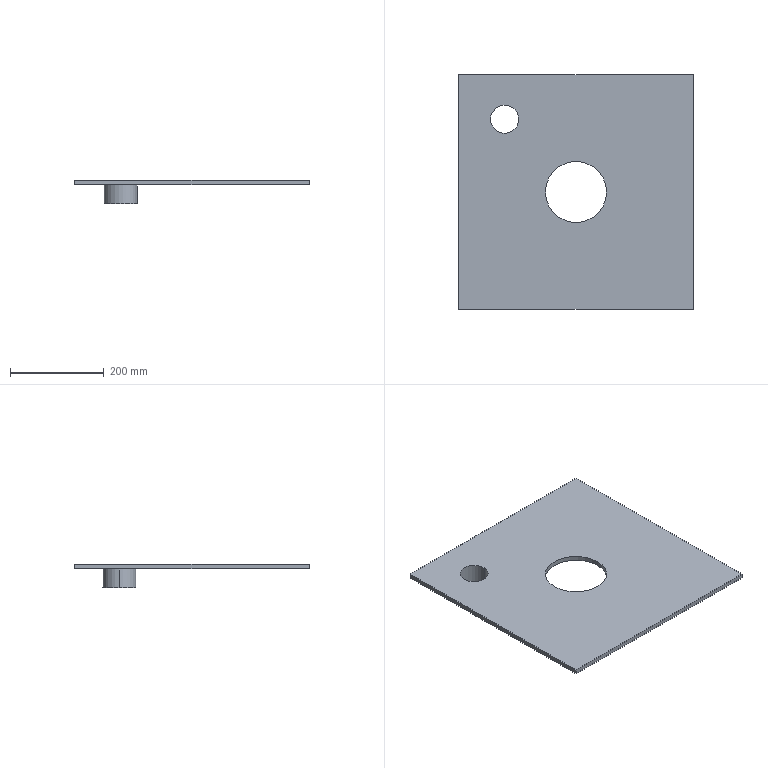Part | SolidWorks | features Extrusion 1, ICE 1 | 1 solid | 13 faces | box 500 x 500 x 50 mm | volume 2380238 mm3 | plane 7 | cylinder 6 | commonest cylinder face diameters 59.914 x2 70 x2 130 x2
STEP:
#1=CARTESIAN_POINT('',(67.956,404.852,-40.));
#2=VERTEX_POINT('',#1);
#3=CARTESIAN_POINT('',(127.871,404.852,-40.));
#4=VERTEX_POINT('',#3);
#5=CARTESIAN_POINT('',(97.914,404.852,-40.));
#6=DIRECTION('',(0.,0.,1.));
#7=DIRECTION('',(1.,0.,0.));
#8=AXIS2_PLACEMENT_3D('',#5,#6,#7);
#9=CIRCLE('',#8,29.957);
#10=EDGE_CURVE('',#2,#4,#9,.T.);
#11=ORIENTED_EDGE('',*,*,#10,.F.);
#12=CARTESIAN_POINT('',(67.956,404.852,10.));
#13=VERTEX_POINT('',#12);
#14=CARTESIAN_POINT('',(67.956,404.852,-40.));
#15=DIRECTION('',(0.,0.,1.));
#16=VECTOR('',#15,1000.);
#17=LINE('',#14,#16);
#18=EDGE_CURVE('',#2,#13,#17,.T.);
#19=ORIENTED_EDGE('',*,*,#18,.T.);
#20=CARTESIAN_POINT('',(127.871,404.852,10.));
#21=VERTEX_POINT('',#20);
#22=CARTESIAN_POINT('',(97.914,404.852,10.));
#23=DIRECTION('',(0.,0.,1.));
#24=DIRECTION('',(1.,0.,0.));
#25=AXIS2_PLACEMENT_3D('',#22,#23,#24);
#26=CIRCLE('',#25,29.957);
#27=EDGE_CURVE('',#13,#21,#26,.T.);
#28=ORIENTED_EDGE('',*,*,#27,.T.);
#29=CARTESIAN_POINT('',(127.871,404.852,-40.));
#30=DIRECTION('',(0.,0.,1.));
#31=VECTOR('',#30,1000.);
#32=LINE('',#29,#31);
#33=EDGE_CURVE('',#4,#21,#32,.T.);
#34=ORIENTED_EDGE('',*,*,#33,.F.);
#35=EDGE_LOOP('',(#11,#19,#28,#34));
#36=FACE_OUTER_BOUND('',#35,.T.);
#37=CARTESIAN_POINT('',(97.914,404.852,-40.));
#38=DIRECTION('',(0.,0.,1.));
#39=DIRECTION('',(1.,0.,0.));
#40=AXIS2_PLACEMENT_3D('',#37,#38,#39);
#41=CYLINDRICAL_SURFACE('',#40,29.957);
#42=ADVANCED_FACE('',(#36),#41,.F.);
#43=CARTESIAN_POINT('',(132.914,404.852,-40.));
#44=VERTEX_POINT('',#43);
#45=CARTESIAN_POINT('',(62.914,404.852,-40.));
#46=VERTEX_POINT('',#45);
#47=CARTESIAN_POINT('',(97.914,404.852,-40.));
#48=DIRECTION('',(0.,0.,1.));
#49=DIRECTION('',(1.,0.,0.));
#50=AXIS2_PLACEMENT_3D('',#47,#48,#49);
#51=CIRCLE('',#50,35.);
#52=EDGE_CURVE('',#44,#46,#51,.T.);
#53=ORIENTED_EDGE('',*,*,#52,.T.);
#54=CARTESIAN_POINT('',(62.914,404.852,0.));
#55=VERTEX_POINT('',#54);
#56=CARTESIAN_POINT('',(62.914,404.852,-40.));
#57=DIRECTION('',(0.,0.,1.));
#58=VECTOR('',#57,1000.);
#59=LINE('',#56,#58);
#60=EDGE_CURVE('',#46,#55,#59,.T.);
#61=ORIENTED_EDGE('',*,*,#60,.T.);
#62=CARTESIAN_POINT('',(132.914,404.852,0.));
#63=VERTEX_POINT('',#62);
#64=CARTESIAN_POINT('',(97.914,404.852,0.));
#65=DIRECTION('',(0.,0.,-1.));
#66=DIRECTION('',(-1.,0.,0.));
#67=AXIS2_PLACEMENT_3D('',#64,#65,#66);
#68=CIRCLE('',#67,35.);
#69=EDGE_CURVE('',#55,#63,#68,.T.);
#70=ORIENTED_EDGE('',*,*,#69,.T.);
#71=CARTESIAN_POINT('',(132.914,404.852,-40.));
#72=DIRECTION('',(0.,0.,1.));
#73=VECTOR('',#72,1000.);
#74=LINE('',#71,#73);
#75=EDGE_CURVE('',#44,#63,#74,.T.);
#76=ORIENTED_EDGE('',*,*,#75,.F.);
#77=EDGE_LOOP('',(#53,#61,#70,#76));
#78=FACE_OUTER_BOUND('',#77,.T.);
#79=CARTESIAN_POINT('',(97.914,404.852,-40.));
#80=DIRECTION('',(0.,0.,1.));
#81=DIRECTION('',(1.,0.,0.));
#82=AXIS2_PLACEMENT_3D('',#79,#80,#81);
#83=CYLINDRICAL_SURFACE('',#82,35.);
#84=ADVANCED_FACE('',(#78),#83,.T.);
#85=CARTESIAN_POINT('',(185.,250.,10.));
#86=VERTEX_POINT('',#85);
#87=CARTESIAN_POINT('',(315.,250.,10.));
#88=VERTEX_POINT('',#87);
#89=CARTESIAN_POINT('',(250.,250.,10.));
#90=DIRECTION('',(0.,0.,1.));
#91=DIRECTION('',(1.,0.,0.));
#92=AXIS2_PLACEMENT_3D('',#89,#90,#91);
#93=CIRCLE('',#92,65.);
#94=EDGE_CURVE('',#86,#88,#93,.T.);
#95=ORIENTED_EDGE('',*,*,#94,.T.);
#96=CARTESIAN_POINT('',(315.,250.,0.));
#97=VERTEX_POINT('',#96);
#98=CARTESIAN_POINT('',(315.,250.,10.));
#99=DIRECTION('',(0.,0.,-1.));
#100=VECTOR('',#99,1000.);
#101=LINE('',#98,#100);
#102=EDGE_CURVE('',#88,#97,#101,.T.);
#103=ORIENTED_EDGE('',*,*,#102,.T.);
#104=CARTESIAN_POINT('',(185.,250.,0.));
#105=VERTEX_POINT('',#104);
#106=CARTESIAN_POINT('',(250.,250.,0.));
#107=DIRECTION('',(0.,0.,1.));
#108=DIRECTION('',(1.,0.,0.));
#109=AXIS2_PLACEMENT_3D('',#106,#107,#108);
#110=CIRCLE('',#109,65.);
#111=EDGE_CURVE('',#105,#97,#110,.T.);
#112=ORIENTED_EDGE('',*,*,#111,.F.);
#113=CARTESIAN_POINT('',(185.,250.,10.));
#114=DIRECTION('',(0.,0.,-1.));
#115=VECTOR('',#114,1000.);
#116=LINE('',#113,#115);
#117=EDGE_CURVE('',#86,#105,#116,.T.);
#118=ORIENTED_EDGE('',*,*,#117,.F.);
#119=EDGE_LOOP('',(#95,#103,#112,#118));
#120=FACE_OUTER_BOUND('',#119,.T.);
#121=CARTESIAN_POINT('',(250.,250.,10.));
#122=DIRECTION('',(0.,0.,-1.));
#123=DIRECTION('',(-1.,0.,0.));
#124=AXIS2_PLACEMENT_3D('',#121,#122,#123);
#125=CYLINDRICAL_SURFACE('',#124,65.);
#126=ADVANCED_FACE('',(#120),#125,.F.);
#127=CARTESIAN_POINT('',(0.,500.,10.));
#128=VERTEX_POINT('',#127);
#129=CARTESIAN_POINT('',(0.,0.,10.));
#130=VERTEX_POINT('',#129);
#131=CARTESIAN_POINT('',(0.,0.,10.));
#132=DIRECTION('',(0.,-1.,0.));
#133=VECTOR('',#132,1000.);
#134=LINE('',#131,#133);
#135=EDGE_CURVE('',#128,#130,#134,.T.);
#136=ORIENTED_EDGE('',*,*,#135,.T.);
#137=CARTESIAN_POINT('',(500.,0.,10.));
#138=VERTEX_POINT('',#137);
#139=CARTESIAN_POINT('',(0.,0.,10.));
#140=DIRECTION('',(1.,0.,0.));
#141=VECTOR('',#140,1000.);
#142=LINE('',#139,#141);
#143=EDGE_CURVE('',#130,#138,#142,.T.);
#144=ORIENTED_EDGE('',*,*,#143,.T.);
#145=CARTESIAN_POINT('',(500.,500.,10.));
#146=VERTEX_POINT('',#145);
#147=CARTESIAN_POINT('',(500.,0.,10.));
#148=DIRECTION('',(0.,1.,0.));
#149=VECTOR('',#148,1000.);
#150=LINE('',#147,#149);
#151=EDGE_CURVE('',#138,#146,#150,.T.);
#152=ORIENTED_EDGE('',*,*,#151,.T.);
#153=CARTESIAN_POINT('',(0.,500.,10.));
#154=DIRECTION('',(-1.,0.,0.));
#155=VECTOR('',#154,1000.);
#156=LINE('',#153,#155);
#157=EDGE_CURVE('',#146,#128,#156,.T.);
#158=ORIENTED_EDGE('',*,*,#157,.T.);
#159=EDGE_LOOP('',(#136,#144,#152,#158));
#160=FACE_OUTER_BOUND('',#159,.T.);
#161=ORIENTED_EDGE('',*,*,#94,.F.);
#162=CARTESIAN_POINT('',(250.,250.,10.));
#163=DIRECTION('',(0.,0.,1.));
#164=DIRECTION('',(1.,0.,0.));
#165=AXIS2_PLACEMENT_3D('',#162,#163,#164);
#166=CIRCLE('',#165,65.);
#167=EDGE_CURVE('',#88,#86,#166,.T.);
#168=ORIENTED_EDGE('',*,*,#167,.F.);
#169=EDGE_LOOP('',(#161,#168));
#170=FACE_BOUND('',#169,.T.);
#171=CARTESIAN_POINT('',(97.914,404.852,10.));
#172=DIRECTION('',(0.,0.,1.));
#173=DIRECTION('',(1.,0.,0.));
#174=AXIS2_PLACEMENT_3D('',#171,#172,#173);
#175=CIRCLE('',#174,29.957);
#176=EDGE_CURVE('',#21,#13,#175,.T.);
#177=ORIENTED_EDGE('',*,*,#176,.F.);
#178=ORIENTED_EDGE('',*,*,#27,.F.);
#179=EDGE_LOOP('',(#177,#178));
#180=FACE_BOUND('',#179,.T.);
#181=CARTESIAN_POINT('',(0.,0.,10.));
#182=DIRECTION('',(0.,0.,-1.));
#183=DIRECTION('',(-1.,0.,0.));
#184=AXIS2_PLACEMENT_3D('',#181,#182,#183);
#185=PLANE('',#184);
#186=ADVANCED_FACE('',(#160,#170,#180),#185,.F.);
#187=CARTESIAN_POINT('',(97.914,404.852,0.));
#188=DIRECTION('',(0.,0.,-1.));
#189=DIRECTION('',(-1.,0.,0.));
#190=AXIS2_PLACEMENT_3D('',#187,#188,#189);
#191=CIRCLE('',#190,35.);
#192=EDGE_CURVE('',#63,#55,#191,.T.);
#193=ORIENTED_EDGE('',*,*,#192,.F.);
#194=ORIENTED_EDGE('',*,*,#69,.F.);
#195=EDGE_LOOP('',(#193,#194));
#196=FACE_BOUND('',#195,.T.);
#197=ORIENTED_EDGE('',*,*,#111,.T.);
#198=CARTESIAN_POINT('',(250.,250.,0.));
#199=DIRECTION('',(0.,0.,1.));
#200=DIRECTION('',(1.,0.,0.));
#201=AXIS2_PLACEMENT_3D('',#198,#199,#200);
#202=CIRCLE('',#201,65.);
#203=EDGE_CURVE('',#97,#105,#202,.T.);
#204=ORIENTED_EDGE('',*,*,#203,.T.);
#205=EDGE_LOOP('',(#197,#204));
#206=FACE_BOUND('',#205,.T.);
#207=CARTESIAN_POINT('',(0.,500.,0.));
#208=VERTEX_POINT('',#207);
#209=CARTESIAN_POINT('',(0.,0.,0.));
#210=VERTEX_POINT('',#209);
#211=CARTESIAN_POINT('',(0.,0.,0.));
#212=DIRECTION('',(0.,-1.,0.));
#213=VECTOR('',#212,1000.);
#214=LINE('',#211,#213);
#215=EDGE_CURVE('',#208,#210,#214,.T.);
#216=ORIENTED_EDGE('',*,*,#215,.F.);
#217=CARTESIAN_POINT('',(500.,500.,0.));
#218=VERTEX_POINT('',#217);
#219=CARTESIAN_POINT('',(0.,500.,0.));
#220=DIRECTION('',(-1.,0.,0.));
#221=VECTOR('',#220,1000.);
#222=LINE('',#219,#221);
#223=EDGE_CURVE('',#218,#208,#222,.T.);
#224=ORIENTED_EDGE('',*,*,#223,.F.);
#225=CARTESIAN_POINT('',(500.,0.,0.));
#226=VERTEX_POINT('',#225);
#227=CARTESIAN_POINT('',(500.,0.,0.));
#228=DIRECTION('',(0.,1.,0.));
#229=VECTOR('',#228,1000.);
#230=LINE('',#227,#229);
#231=EDGE_CURVE('',#226,#218,#230,.T.);
#232=ORIENTED_EDGE('',*,*,#231,.F.);
#233=CARTESIAN_POINT('',(0.,0.,0.));
#234=DIRECTION('',(1.,0.,0.));
#235=VECTOR('',#234,1000.);
#236=LINE('',#233,#235);
#237=EDGE_CURVE('',#210,#226,#236,.T.);
#238=ORIENTED_EDGE('',*,*,#237,.F.);
#239=EDGE_LOOP('',(#216,#224,#232,#238));
#240=FACE_OUTER_BOUND('',#239,.T.);
#241=CARTESIAN_POINT('',(0.,0.,0.));
#242=DIRECTION('',(0.,0.,-1.));
#243=DIRECTION('',(-1.,0.,0.));
#244=AXIS2_PLACEMENT_3D('',#241,#242,#243);
#245=PLANE('',#244);
#246=ADVANCED_FACE('',(#196,#206,#240),#245,.T.);
#247=ORIENTED_EDGE('',*,*,#215,.T.);
#248=CARTESIAN_POINT('',(0.,0.,10.));
#249=DIRECTION('',(0.,0.,-1.));
#250=VECTOR('',#249,1000.);
#251=LINE('',#248,#250);
#252=EDGE_CURVE('',#130,#210,#251,.T.);
#253=ORIENTED_EDGE('',*,*,#252,.F.);
#254=ORIENTED_EDGE('',*,*,#135,.F.);
#255=CARTESIAN_POINT('',(0.,500.,10.));
#256=DIRECTION('',(0.,0.,-1.));
#257=VECTOR('',#256,1000.);
#258=LINE('',#255,#257);
#259=EDGE_CURVE('',#128,#208,#258,.T.);
#260=ORIENTED_EDGE('',*,*,#259,.T.);
#261=EDGE_LOOP('',(#247,#253,#254,#260));
#262=FACE_OUTER_BOUND('',#261,.T.);
#263=CARTESIAN_POINT('',(0.,0.,10.));
#264=DIRECTION('',(1.,0.,0.));
#265=DIRECTION('',(0.,0.,-1.));
#266=AXIS2_PLACEMENT_3D('',#263,#264,#265);
#267=PLANE('',#266);
#268=ADVANCED_FACE('',(#262),#267,.F.);
#269=ORIENTED_EDGE('',*,*,#237,.T.);
#270=CARTESIAN_POINT('',(500.,0.,10.));
#271=DIRECTION('',(0.,0.,-1.));
#272=VECTOR('',#271,1000.);
#273=LINE('',#270,#272);
#274=EDGE_CURVE('',#138,#226,#273,.T.);
#275=ORIENTED_EDGE('',*,*,#274,.F.);
#276=ORIENTED_EDGE('',*,*,#143,.F.);
#277=ORIENTED_EDGE('',*,*,#252,.T.);
#278=EDGE_LOOP('',(#269,#275,#276,#277));
#279=FACE_OUTER_BOUND('',#278,.T.);
#280=CARTESIAN_POINT('',(0.,0.,10.));
#281=DIRECTION('',(0.,1.,0.));
#282=DIRECTION('',(0.,0.,1.));
#283=AXIS2_PLACEMENT_3D('',#280,#281,#282);
#284=PLANE('',#283);
#285=ADVANCED_FACE('',(#279),#284,.F.);
#286=ORIENTED_EDGE('',*,*,#231,.T.);
#287=CARTESIAN_POINT('',(500.,500.,10.));
#288=DIRECTION('',(0.,0.,-1.));
#289=VECTOR('',#288,1000.);
#290=LINE('',#287,#289);
#291=EDGE_CURVE('',#146,#218,#290,.T.);
#292=ORIENTED_EDGE('',*,*,#291,.F.);
#293=ORIENTED_EDGE('',*,*,#151,.F.);
#294=ORIENTED_EDGE('',*,*,#274,.T.);
#295=EDGE_LOOP('',(#286,#292,#293,#294));
#296=FACE_OUTER_BOUND('',#295,.T.);
#297=CARTESIAN_POINT('',(500.,0.,10.));
#298=DIRECTION('',(-1.,0.,0.));
#299=DIRECTION('',(0.,0.,1.));
#300=AXIS2_PLACEMENT_3D('',#297,#298,#299);
#301=PLANE('',#300);
#302=ADVANCED_FACE('',(#296),#301,.F.);
#303=ORIENTED_EDGE('',*,*,#223,.T.);
#304=ORIENTED_EDGE('',*,*,#259,.F.);
#305=ORIENTED_EDGE('',*,*,#157,.F.);
#306=ORIENTED_EDGE('',*,*,#291,.T.);
#307=EDGE_LOOP('',(#303,#304,#305,#306));
#308=FACE_OUTER_BOUND('',#307,.T.);
#309=CARTESIAN_POINT('',(0.,500.,10.));
#310=DIRECTION('',(0.,-1.,0.));
#311=DIRECTION('',(0.,0.,-1.));
#312=AXIS2_PLACEMENT_3D('',#309,#310,#311);
#313=PLANE('',#312);
#314=ADVANCED_FACE('',(#308),#313,.F.);
#315=ORIENTED_EDGE('',*,*,#102,.F.);
#316=ORIENTED_EDGE('',*,*,#167,.T.);
#317=ORIENTED_EDGE('',*,*,#117,.T.);
#318=ORIENTED_EDGE('',*,*,#203,.F.);
#319=EDGE_LOOP('',(#315,#316,#317,#318));
#320=FACE_OUTER_BOUND('',#319,.T.);
#321=CARTESIAN_POINT('',(250.,250.,10.));
#322=DIRECTION('',(0.,0.,-1.));
#323=DIRECTION('',(-1.,0.,0.));
#324=AXIS2_PLACEMENT_3D('',#321,#322,#323);
#325=CYLINDRICAL_SURFACE('',#324,65.);
#326=ADVANCED_FACE('',(#320),#325,.F.);
#327=ORIENTED_EDGE('',*,*,#60,.F.);
#328=CARTESIAN_POINT('',(97.914,404.852,-40.));
#329=DIRECTION('',(0.,0.,1.));
#330=DIRECTION('',(1.,0.,0.));
#331=AXIS2_PLACEMENT_3D('',#328,#329,#330);
#332=CIRCLE('',#331,35.);
#333=EDGE_CURVE('',#46,#44,#332,.T.);
#334=ORIENTED_EDGE('',*,*,#333,.T.);
#335=ORIENTED_EDGE('',*,*,#75,.T.);
#336=ORIENTED_EDGE('',*,*,#192,.T.);
#337=EDGE_LOOP('',(#327,#334,#335,#336));
#338=FACE_OUTER_BOUND('',#337,.T.);
#339=CARTESIAN_POINT('',(97.914,404.852,-40.));
#340=DIRECTION('',(0.,0.,1.));
#341=DIRECTION('',(1.,0.,0.));
#342=AXIS2_PLACEMENT_3D('',#339,#340,#341);
#343=CYLINDRICAL_SURFACE('',#342,35.);
#344=ADVANCED_FACE('',(#338),#343,.T.);
#345=CARTESIAN_POINT('',(97.914,404.852,-40.));
#346=DIRECTION('',(0.,0.,1.));
#347=DIRECTION('',(1.,0.,0.));
#348=AXIS2_PLACEMENT_3D('',#345,#346,#347);
#349=CIRCLE('',#348,29.957);
#350=EDGE_CURVE('',#4,#2,#349,.T.);
#351=ORIENTED_EDGE('',*,*,#350,.T.);
#352=ORIENTED_EDGE('',*,*,#10,.T.);
#353=EDGE_LOOP('',(#351,#352));
#354=FACE_BOUND('',#353,.T.);
#355=ORIENTED_EDGE('',*,*,#52,.F.);
#356=ORIENTED_EDGE('',*,*,#333,.F.);
#357=EDGE_LOOP('',(#355,#356));
#358=FACE_OUTER_BOUND('',#357,.T.);
#359=CARTESIAN_POINT('',(97.914,404.852,-40.));
#360=DIRECTION('',(0.,0.,1.));
#361=DIRECTION('',(1.,0.,0.));
#362=AXIS2_PLACEMENT_3D('',#359,#360,#361);
#363=PLANE('',#362);
#364=ADVANCED_FACE('',(#354,#358),#363,.F.);
#365=ORIENTED_EDGE('',*,*,#18,.F.);
#366=ORIENTED_EDGE('',*,*,#350,.F.);
#367=ORIENTED_EDGE('',*,*,#33,.T.);
#368=ORIENTED_EDGE('',*,*,#176,.T.);
#369=EDGE_LOOP('',(#365,#366,#367,#368));
#370=FACE_OUTER_BOUND('',#369,.T.);
#371=CARTESIAN_POINT('',(97.914,404.852,-40.));
#372=DIRECTION('',(0.,0.,1.));
#373=DIRECTION('',(1.,0.,0.));
#374=AXIS2_PLACEMENT_3D('',#371,#372,#373);
#375=CYLINDRICAL_SURFACE('',#374,29.957);
#376=ADVANCED_FACE('',(#370),#375,.F.);
#377=CLOSED_SHELL('',(#42,#84,#126,#186,#246,#268,#285,#302,#314,#326,#344,#364,#376));
#378=MANIFOLD_SOLID_BREP('',#377);
#379=CARTESIAN_POINT('',(0.,0.,0.));
#380=DIRECTION('',(0.,0.,1.));
#381=DIRECTION('',(1.,0.,0.));
#382=AXIS2_PLACEMENT_3D('',#379,#380,#381);
#383=(LENGTH_UNIT()NAMED_UNIT(*)SI_UNIT(.MILLI.,.METRE.));
#384=UNCERTAINTY_MEASURE_WITH_UNIT(LENGTH_MEASURE(0.00001),#383,'','');
#385=(NAMED_UNIT(*)PLANE_ANGLE_UNIT()SI_UNIT($,.RADIAN.));
#386=(NAMED_UNIT(*)SI_UNIT($,.STERADIAN.)SOLID_ANGLE_UNIT());
#387=(GEOMETRIC_REPRESENTATION_CONTEXT(3)GLOBAL_UNCERTAINTY_ASSIGNED_CONTEXT((#384))GLOBAL_UNIT_ASSIGNED_CONTEXT((#383,#385,#386))REPRESENTATION_CONTEXT('',''));
#388=ADVANCED_BREP_SHAPE_REPRESENTATION('',(#378,#382),#387);